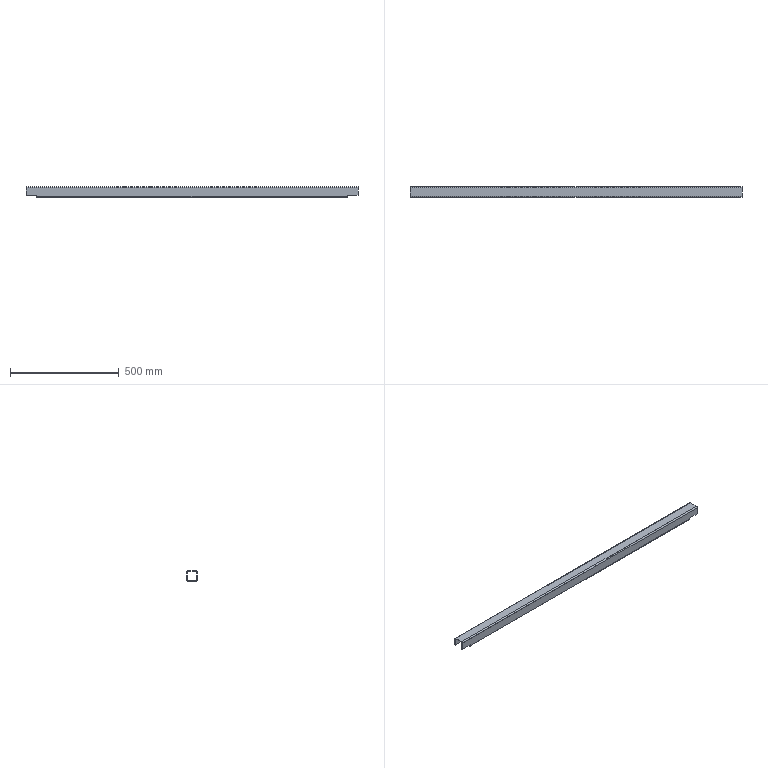Part | SolidWorks | features BaseBody 1 | 1 solid | 89 faces | box 1530 x 50 x 50 mm | volume 809268 mm3 | plane 36 | spline 35 | cylinder 18 | commonest cylinder face diameters 3.3 x10 6 x4 12 x4